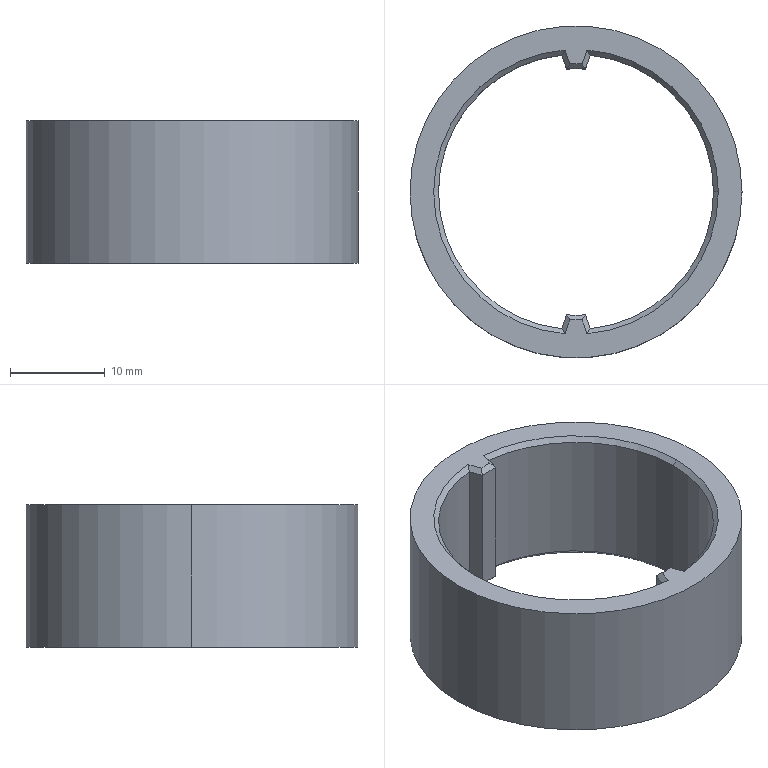Part | SolidWorks | features Chamfer 1, Extrusion 1, ICE 1 | 1 solid | 31 faces | box 35 x 35 x 15 mm | volume 4612 mm3 | plane 14 | cone 10 | cylinder 7 | commonest cylinder face diameters 29 x3 26 x2 35 x2
STEP:
#1=CARTESIAN_POINT('',(14.5,0.,14.5));
#2=VERTEX_POINT('',#1);
#3=CARTESIAN_POINT('',(1.5,14.422,14.5));
#4=VERTEX_POINT('',#3);
#5=CARTESIAN_POINT('',(0.,0.,14.5));
#6=DIRECTION('',(0.,0.,1.));
#7=DIRECTION('',(1.,0.,0.));
#8=AXIS2_PLACEMENT_3D('',#5,#6,#7);
#9=CIRCLE('',#8,14.5);
#10=EDGE_CURVE('',#2,#4,#9,.T.);
#11=ORIENTED_EDGE('',*,*,#10,.F.);
#12=CARTESIAN_POINT('',(15.,0.,15.));
#13=VERTEX_POINT('',#12);
#14=CARTESIAN_POINT('',(14.5,0.,14.5));
#15=DIRECTION('',(0.7071,0.,0.7071));
#16=VECTOR('',#15,1000.);
#17=LINE('',#14,#16);
#18=EDGE_CURVE('',#2,#13,#17,.T.);
#19=ORIENTED_EDGE('',*,*,#18,.T.);
#20=CARTESIAN_POINT('',(1.154,14.956,15.));
#21=VERTEX_POINT('',#20);
#22=CARTESIAN_POINT('',(0.,0.,15.));
#23=DIRECTION('',(0.,0.,-1.));
#24=DIRECTION('',(1.,0.,0.));
#25=AXIS2_PLACEMENT_3D('',#22,#23,#24);
#26=CIRCLE('',#25,15.);
#27=EDGE_CURVE('',#21,#13,#26,.T.);
#28=ORIENTED_EDGE('',*,*,#27,.F.);
#29=CARTESIAN_POINT('',(1.154,14.956,15.));
#30=CARTESIAN_POINT('',(1.27,14.779,14.833));
#31=CARTESIAN_POINT('',(1.386,14.601,14.666));
#32=CARTESIAN_POINT('',(1.5,14.422,14.5));
#33=B_SPLINE_CURVE_WITH_KNOTS('',3,(#29,#30,#31,#32),.UNSPECIFIED.,.F.,.F.,(4,4),(0.,0.0008088),.UNSPECIFIED.);
#34=EDGE_CURVE('',#21,#4,#33,.T.);
#35=ORIENTED_EDGE('',*,*,#34,.T.);
#36=EDGE_LOOP('',(#11,#19,#28,#35));
#37=FACE_OUTER_BOUND('',#36,.T.);
#38=CARTESIAN_POINT('',(0.,0.,14.5));
#39=DIRECTION('',(0.,0.,1.));
#40=DIRECTION('',(1.,0.,0.));
#41=AXIS2_PLACEMENT_3D('',#38,#39,#40);
#42=CONICAL_SURFACE('',#41,14.5,0.7854);
#43=ADVANCED_FACE('',(#37),#42,.F.);
#44=CARTESIAN_POINT('',(-14.5,0.,0.5));
#45=VERTEX_POINT('',#44);
#46=CARTESIAN_POINT('',(-1.5,14.422,0.5));
#47=VERTEX_POINT('',#46);
#48=CARTESIAN_POINT('',(0.,0.,0.5));
#49=DIRECTION('',(0.,0.,-1.));
#50=DIRECTION('',(1.,0.,0.));
#51=AXIS2_PLACEMENT_3D('',#48,#49,#50);
#52=CIRCLE('',#51,14.5);
#53=EDGE_CURVE('',#45,#47,#52,.T.);
#54=ORIENTED_EDGE('',*,*,#53,.F.);
#55=CARTESIAN_POINT('',(-15.,0.,0.));
#56=VERTEX_POINT('',#55);
#57=CARTESIAN_POINT('',(-15.,0.,0.));
#58=DIRECTION('',(-0.7071,0.,-0.7071));
#59=VECTOR('',#58,1000.);
#60=LINE('',#57,#59);
#61=EDGE_CURVE('',#45,#56,#60,.T.);
#62=ORIENTED_EDGE('',*,*,#61,.T.);
#63=CARTESIAN_POINT('',(-1.154,14.956,0.));
#64=VERTEX_POINT('',#63);
#65=CARTESIAN_POINT('',(0.,0.,0.));
#66=DIRECTION('',(0.,0.,1.));
#67=DIRECTION('',(1.,0.,0.));
#68=AXIS2_PLACEMENT_3D('',#65,#66,#67);
#69=CIRCLE('',#68,15.);
#70=EDGE_CURVE('',#64,#56,#69,.T.);
#71=ORIENTED_EDGE('',*,*,#70,.F.);
#72=CARTESIAN_POINT('',(-1.154,14.956,0.));
#73=CARTESIAN_POINT('',(-1.27,14.779,0.1672));
#74=CARTESIAN_POINT('',(-1.386,14.601,0.3339));
#75=CARTESIAN_POINT('',(-1.5,14.422,0.5));
#76=B_SPLINE_CURVE_WITH_KNOTS('',3,(#72,#73,#74,#75),.UNSPECIFIED.,.F.,.F.,(4,4),(0.,0.0008088),.UNSPECIFIED.);
#77=EDGE_CURVE('',#64,#47,#76,.T.);
#78=ORIENTED_EDGE('',*,*,#77,.T.);
#79=EDGE_LOOP('',(#54,#62,#71,#78));
#80=FACE_OUTER_BOUND('',#79,.T.);
#81=CARTESIAN_POINT('',(0.,0.,0.));
#82=DIRECTION('',(0.,0.,-1.));
#83=DIRECTION('',(-1.,0.,0.));
#84=AXIS2_PLACEMENT_3D('',#81,#82,#83);
#85=CONICAL_SURFACE('',#84,15.,0.7854);
#86=ADVANCED_FACE('',(#80),#85,.F.);
#87=CARTESIAN_POINT('',(17.5,0.,15.));
#88=VERTEX_POINT('',#87);
#89=CARTESIAN_POINT('',(-17.5,0.,15.));
#90=VERTEX_POINT('',#89);
#91=CARTESIAN_POINT('',(0.,0.,15.));
#92=DIRECTION('',(0.,0.,1.));
#93=DIRECTION('',(1.,0.,0.));
#94=AXIS2_PLACEMENT_3D('',#91,#92,#93);
#95=CIRCLE('',#94,17.5);
#96=EDGE_CURVE('',#88,#90,#95,.T.);
#97=ORIENTED_EDGE('',*,*,#96,.F.);
#98=CARTESIAN_POINT('',(17.5,0.,0.));
#99=VERTEX_POINT('',#98);
#100=CARTESIAN_POINT('',(17.5,0.,15.));
#101=DIRECTION('',(0.,0.,-1.));
#102=VECTOR('',#101,1000.);
#103=LINE('',#100,#102);
#104=EDGE_CURVE('',#88,#99,#103,.T.);
#105=ORIENTED_EDGE('',*,*,#104,.T.);
#106=CARTESIAN_POINT('',(-17.5,0.,0.));
#107=VERTEX_POINT('',#106);
#108=CARTESIAN_POINT('',(0.,0.,0.));
#109=DIRECTION('',(0.,0.,1.));
#110=DIRECTION('',(1.,0.,0.));
#111=AXIS2_PLACEMENT_3D('',#108,#109,#110);
#112=CIRCLE('',#111,17.5);
#113=EDGE_CURVE('',#99,#107,#112,.T.);
#114=ORIENTED_EDGE('',*,*,#113,.T.);
#115=CARTESIAN_POINT('',(-17.5,0.,15.));
#116=DIRECTION('',(0.,0.,-1.));
#117=VECTOR('',#116,1000.);
#118=LINE('',#115,#117);
#119=EDGE_CURVE('',#90,#107,#118,.T.);
#120=ORIENTED_EDGE('',*,*,#119,.F.);
#121=EDGE_LOOP('',(#97,#105,#114,#120));
#122=FACE_OUTER_BOUND('',#121,.T.);
#123=CARTESIAN_POINT('',(0.,0.,15.));
#124=DIRECTION('',(0.,0.,-1.));
#125=DIRECTION('',(-1.,0.,0.));
#126=AXIS2_PLACEMENT_3D('',#123,#124,#125);
#127=CYLINDRICAL_SURFACE('',#126,17.5);
#128=ADVANCED_FACE('',(#122),#127,.T.);
#129=CARTESIAN_POINT('',(-1.5,14.422,14.5));
#130=VERTEX_POINT('',#129);
#131=CARTESIAN_POINT('',(-14.5,0.,14.5));
#132=VERTEX_POINT('',#131);
#133=CARTESIAN_POINT('',(0.,0.,14.5));
#134=DIRECTION('',(0.,0.,1.));
#135=DIRECTION('',(1.,0.,0.));
#136=AXIS2_PLACEMENT_3D('',#133,#134,#135);
#137=CIRCLE('',#136,14.5);
#138=EDGE_CURVE('',#130,#132,#137,.T.);
#139=ORIENTED_EDGE('',*,*,#138,.T.);
#140=CARTESIAN_POINT('',(-14.5,0.,15.));
#141=DIRECTION('',(0.,0.,-1.));
#142=VECTOR('',#141,1000.);
#143=LINE('',#140,#142);
#144=EDGE_CURVE('',#132,#45,#143,.T.);
#145=ORIENTED_EDGE('',*,*,#144,.T.);
#146=ORIENTED_EDGE('',*,*,#53,.T.);
#147=CARTESIAN_POINT('',(-1.5,14.422,18.372));
#148=DIRECTION('',(0.,0.,-1.));
#149=VECTOR('',#148,1000.);
#150=LINE('',#147,#149);
#151=EDGE_CURVE('',#130,#47,#150,.T.);
#152=ORIENTED_EDGE('',*,*,#151,.F.);
#153=EDGE_LOOP('',(#139,#145,#146,#152));
#154=FACE_OUTER_BOUND('',#153,.T.);
#155=CARTESIAN_POINT('',(0.,0.,15.));
#156=DIRECTION('',(0.,0.,-1.));
#157=DIRECTION('',(-1.,0.,0.));
#158=AXIS2_PLACEMENT_3D('',#155,#156,#157);
#159=CYLINDRICAL_SURFACE('',#158,14.5);
#160=ADVANCED_FACE('',(#154),#159,.F.);
#161=CARTESIAN_POINT('',(1.5,14.422,0.5));
#162=VERTEX_POINT('',#161);
#163=CARTESIAN_POINT('',(1.5,14.422,18.372));
#164=DIRECTION('',(0.,0.,-1.));
#165=VECTOR('',#164,1000.);
#166=LINE('',#163,#165);
#167=EDGE_CURVE('',#4,#162,#166,.T.);
#168=ORIENTED_EDGE('',*,*,#167,.T.);
#169=CARTESIAN_POINT('',(1.5,-14.422,0.5));
#170=VERTEX_POINT('',#169);
#171=CARTESIAN_POINT('',(0.,0.,0.5));
#172=DIRECTION('',(0.,0.,-1.));
#173=DIRECTION('',(1.,0.,0.));
#174=AXIS2_PLACEMENT_3D('',#171,#172,#173);
#175=CIRCLE('',#174,14.5);
#176=EDGE_CURVE('',#162,#170,#175,.T.);
#177=ORIENTED_EDGE('',*,*,#176,.T.);
#178=CARTESIAN_POINT('',(1.5,-14.422,14.5));
#179=VERTEX_POINT('',#178);
#180=CARTESIAN_POINT('',(1.5,-14.422,18.372));
#181=DIRECTION('',(0.,0.,-1.));
#182=VECTOR('',#181,1000.);
#183=LINE('',#180,#182);
#184=EDGE_CURVE('',#179,#170,#183,.T.);
#185=ORIENTED_EDGE('',*,*,#184,.F.);
#186=CARTESIAN_POINT('',(0.,0.,14.5));
#187=DIRECTION('',(0.,0.,1.));
#188=DIRECTION('',(1.,0.,0.));
#189=AXIS2_PLACEMENT_3D('',#186,#187,#188);
#190=CIRCLE('',#189,14.5);
#191=EDGE_CURVE('',#179,#2,#190,.T.);
#192=ORIENTED_EDGE('',*,*,#191,.T.);
#193=ORIENTED_EDGE('',*,*,#10,.T.);
#194=EDGE_LOOP('',(#168,#177,#185,#192,#193));
#195=FACE_OUTER_BOUND('',#194,.T.);
#196=CARTESIAN_POINT('',(0.,0.,15.));
#197=DIRECTION('',(0.,0.,-1.));
#198=DIRECTION('',(-1.,0.,0.));
#199=AXIS2_PLACEMENT_3D('',#196,#197,#198);
#200=CYLINDRICAL_SURFACE('',#199,14.5);
#201=ADVANCED_FACE('',(#195),#200,.F.);
#202=ORIENTED_EDGE('',*,*,#144,.F.);
#203=CARTESIAN_POINT('',(-1.5,-14.422,14.5));
#204=VERTEX_POINT('',#203);
#205=CARTESIAN_POINT('',(0.,0.,14.5));
#206=DIRECTION('',(0.,0.,1.));
#207=DIRECTION('',(1.,0.,0.));
#208=AXIS2_PLACEMENT_3D('',#205,#206,#207);
#209=CIRCLE('',#208,14.5);
#210=EDGE_CURVE('',#132,#204,#209,.T.);
#211=ORIENTED_EDGE('',*,*,#210,.T.);
#212=CARTESIAN_POINT('',(-1.5,-14.422,0.5));
#213=VERTEX_POINT('',#212);
#214=CARTESIAN_POINT('',(-1.5,-14.422,18.372));
#215=DIRECTION('',(0.,0.,-1.));
#216=VECTOR('',#215,1000.);
#217=LINE('',#214,#216);
#218=EDGE_CURVE('',#204,#213,#217,.T.);
#219=ORIENTED_EDGE('',*,*,#218,.T.);
#220=CARTESIAN_POINT('',(0.,0.,0.5));
#221=DIRECTION('',(0.,0.,-1.));
#222=DIRECTION('',(1.,0.,0.));
#223=AXIS2_PLACEMENT_3D('',#220,#221,#222);
#224=CIRCLE('',#223,14.5);
#225=EDGE_CURVE('',#213,#45,#224,.T.);
#226=ORIENTED_EDGE('',*,*,#225,.T.);
#227=EDGE_LOOP('',(#202,#211,#219,#226));
#228=FACE_OUTER_BOUND('',#227,.T.);
#229=CARTESIAN_POINT('',(0.,0.,15.));
#230=DIRECTION('',(0.,0.,-1.));
#231=DIRECTION('',(-1.,0.,0.));
#232=AXIS2_PLACEMENT_3D('',#229,#230,#231);
#233=CYLINDRICAL_SURFACE('',#232,14.5);
#234=ADVANCED_FACE('',(#228),#233,.F.);
#235=CARTESIAN_POINT('',(1.154,-14.956,15.));
#236=VERTEX_POINT('',#235);
#237=CARTESIAN_POINT('',(0.6505,-13.484,15.));
#238=VERTEX_POINT('',#237);
#239=CARTESIAN_POINT('',(0.5269,-13.123,15.));
#240=DIRECTION('',(-0.3238,0.9461,0.));
#241=VECTOR('',#240,1000.);
#242=LINE('',#239,#241);
#243=EDGE_CURVE('',#236,#238,#242,.T.);
#244=ORIENTED_EDGE('',*,*,#243,.T.);
#245=CARTESIAN_POINT('',(-0.6505,-13.484,15.));
#246=VERTEX_POINT('',#245);
#247=CARTESIAN_POINT('',(0.,0.,15.));
#248=DIRECTION('',(0.,0.,-1.));
#249=DIRECTION('',(1.,0.,0.));
#250=AXIS2_PLACEMENT_3D('',#247,#248,#249);
#251=CIRCLE('',#250,13.5);
#252=EDGE_CURVE('',#238,#246,#251,.T.);
#253=ORIENTED_EDGE('',*,*,#252,.T.);
#254=CARTESIAN_POINT('',(-1.154,-14.956,15.));
#255=VERTEX_POINT('',#254);
#256=CARTESIAN_POINT('',(-1.027,-14.584,15.));
#257=DIRECTION('',(-0.3238,-0.9461,0.));
#258=VECTOR('',#257,1000.);
#259=LINE('',#256,#258);
#260=EDGE_CURVE('',#246,#255,#259,.T.);
#261=ORIENTED_EDGE('',*,*,#260,.T.);
#262=CARTESIAN_POINT('',(-1.154,14.956,15.));
#263=VERTEX_POINT('',#262);
#264=CARTESIAN_POINT('',(0.,0.,15.));
#265=DIRECTION('',(0.,0.,-1.));
#266=DIRECTION('',(1.,0.,0.));
#267=AXIS2_PLACEMENT_3D('',#264,#265,#266);
#268=CIRCLE('',#267,15.);
#269=EDGE_CURVE('',#255,#263,#268,.T.);
#270=ORIENTED_EDGE('',*,*,#269,.T.);
#271=CARTESIAN_POINT('',(-0.6505,13.484,15.));
#272=VERTEX_POINT('',#271);
#273=CARTESIAN_POINT('',(-0.5269,13.123,15.));
#274=DIRECTION('',(0.3238,-0.9461,0.));
#275=VECTOR('',#274,1000.);
#276=LINE('',#273,#275);
#277=EDGE_CURVE('',#263,#272,#276,.T.);
#278=ORIENTED_EDGE('',*,*,#277,.T.);
#279=CARTESIAN_POINT('',(0.6505,13.484,15.));
#280=VERTEX_POINT('',#279);
#281=CARTESIAN_POINT('',(0.,0.,15.));
#282=DIRECTION('',(0.,0.,-1.));
#283=DIRECTION('',(1.,0.,0.));
#284=AXIS2_PLACEMENT_3D('',#281,#282,#283);
#285=CIRCLE('',#284,13.5);
#286=EDGE_CURVE('',#272,#280,#285,.T.);
#287=ORIENTED_EDGE('',*,*,#286,.T.);
#288=CARTESIAN_POINT('',(1.027,14.584,15.));
#289=DIRECTION('',(0.3238,0.9461,0.));
#290=VECTOR('',#289,1000.);
#291=LINE('',#288,#290);
#292=EDGE_CURVE('',#280,#21,#291,.T.);
#293=ORIENTED_EDGE('',*,*,#292,.T.);
#294=ORIENTED_EDGE('',*,*,#27,.T.);
#295=CARTESIAN_POINT('',(0.,0.,15.));
#296=DIRECTION('',(0.,0.,-1.));
#297=DIRECTION('',(1.,0.,0.));
#298=AXIS2_PLACEMENT_3D('',#295,#296,#297);
#299=CIRCLE('',#298,15.);
#300=EDGE_CURVE('',#13,#236,#299,.T.);
#301=ORIENTED_EDGE('',*,*,#300,.T.);
#302=EDGE_LOOP('',(#244,#253,#261,#270,#278,#287,#293,#294,#301));
#303=FACE_BOUND('',#302,.T.);
#304=CARTESIAN_POINT('',(0.,0.,15.));
#305=DIRECTION('',(0.,0.,1.));
#306=DIRECTION('',(1.,0.,0.));
#307=AXIS2_PLACEMENT_3D('',#304,#305,#306);
#308=CIRCLE('',#307,17.5);
#309=EDGE_CURVE('',#90,#88,#308,.T.);
#310=ORIENTED_EDGE('',*,*,#309,.T.);
#311=ORIENTED_EDGE('',*,*,#96,.T.);
#312=EDGE_LOOP('',(#310,#311));
#313=FACE_OUTER_BOUND('',#312,.T.);
#314=CARTESIAN_POINT('',(0.,0.,15.));
#315=DIRECTION('',(0.,0.,1.));
#316=DIRECTION('',(1.,0.,0.));
#317=AXIS2_PLACEMENT_3D('',#314,#315,#316);
#318=PLANE('',#317);
#319=ADVANCED_FACE('',(#303,#313),#318,.T.);
#320=CARTESIAN_POINT('',(-1.154,-14.956,0.));
#321=VERTEX_POINT('',#320);
#322=CARTESIAN_POINT('',(-0.6505,-13.484,0.));
#323=VERTEX_POINT('',#322);
#324=CARTESIAN_POINT('',(3.549,-1.215,0.));
#325=DIRECTION('',(0.3238,0.9461,0.));
#326=VECTOR('',#325,1000.);
#327=LINE('',#324,#326);
#328=EDGE_CURVE('',#321,#323,#327,.T.);
#329=ORIENTED_EDGE('',*,*,#328,.T.);
#330=CARTESIAN_POINT('',(0.6505,-13.484,0.));
#331=VERTEX_POINT('',#330);
#332=CARTESIAN_POINT('',(0.,0.,0.));
#333=DIRECTION('',(0.,0.,1.));
#334=DIRECTION('',(1.,0.,0.));
#335=AXIS2_PLACEMENT_3D('',#332,#333,#334);
#336=CIRCLE('',#335,13.5);
#337=EDGE_CURVE('',#323,#331,#336,.T.);
#338=ORIENTED_EDGE('',*,*,#337,.T.);
#339=CARTESIAN_POINT('',(1.154,-14.956,0.));
#340=VERTEX_POINT('',#339);
#341=CARTESIAN_POINT('',(-3.549,-1.215,0.));
#342=DIRECTION('',(0.3238,-0.9461,0.));
#343=VECTOR('',#342,1000.);
#344=LINE('',#341,#343);
#345=EDGE_CURVE('',#331,#340,#344,.T.);
#346=ORIENTED_EDGE('',*,*,#345,.T.);
#347=CARTESIAN_POINT('',(1.154,14.956,0.));
#348=VERTEX_POINT('',#347);
#349=CARTESIAN_POINT('',(0.,0.,0.));
#350=DIRECTION('',(0.,0.,1.));
#351=DIRECTION('',(1.,0.,0.));
#352=AXIS2_PLACEMENT_3D('',#349,#350,#351);
#353=CIRCLE('',#352,15.);
#354=EDGE_CURVE('',#340,#348,#353,.T.);
#355=ORIENTED_EDGE('',*,*,#354,.T.);
#356=CARTESIAN_POINT('',(0.6505,13.484,0.));
#357=VERTEX_POINT('',#356);
#358=CARTESIAN_POINT('',(-3.549,1.215,0.));
#359=DIRECTION('',(-0.3238,-0.9461,0.));
#360=VECTOR('',#359,1000.);
#361=LINE('',#358,#360);
#362=EDGE_CURVE('',#348,#357,#361,.T.);
#363=ORIENTED_EDGE('',*,*,#362,.T.);
#364=CARTESIAN_POINT('',(-0.6505,13.484,0.));
#365=VERTEX_POINT('',#364);
#366=CARTESIAN_POINT('',(0.,0.,0.));
#367=DIRECTION('',(0.,0.,1.));
#368=DIRECTION('',(1.,0.,0.));
#369=AXIS2_PLACEMENT_3D('',#366,#367,#368);
#370=CIRCLE('',#369,13.5);
#371=EDGE_CURVE('',#357,#365,#370,.T.);
#372=ORIENTED_EDGE('',*,*,#371,.T.);
#373=CARTESIAN_POINT('',(3.549,1.215,0.));
#374=DIRECTION('',(-0.3238,0.9461,0.));
#375=VECTOR('',#374,1000.);
#376=LINE('',#373,#375);
#377=EDGE_CURVE('',#365,#64,#376,.T.);
#378=ORIENTED_EDGE('',*,*,#377,.T.);
#379=ORIENTED_EDGE('',*,*,#70,.T.);
#380=CARTESIAN_POINT('',(0.,0.,0.));
#381=DIRECTION('',(0.,0.,1.));
#382=DIRECTION('',(1.,0.,0.));
#383=AXIS2_PLACEMENT_3D('',#380,#381,#382);
#384=CIRCLE('',#383,15.);
#385=EDGE_CURVE('',#56,#321,#384,.T.);
#386=ORIENTED_EDGE('',*,*,#385,.T.);
#387=EDGE_LOOP('',(#329,#338,#346,#355,#363,#372,#378,#379,#386));
#388=FACE_BOUND('',#387,.T.);
#389=CARTESIAN_POINT('',(0.,0.,0.));
#390=DIRECTION('',(0.,0.,1.));
#391=DIRECTION('',(1.,0.,0.));
#392=AXIS2_PLACEMENT_3D('',#389,#390,#391);
#393=CIRCLE('',#392,17.5);
#394=EDGE_CURVE('',#107,#99,#393,.T.);
#395=ORIENTED_EDGE('',*,*,#394,.F.);
#396=ORIENTED_EDGE('',*,*,#113,.F.);
#397=EDGE_LOOP('',(#395,#396));
#398=FACE_OUTER_BOUND('',#397,.T.);
#399=CARTESIAN_POINT('',(0.,0.,0.));
#400=DIRECTION('',(0.,0.,1.));
#401=DIRECTION('',(1.,0.,0.));
#402=AXIS2_PLACEMENT_3D('',#399,#400,#401);
#403=PLANE('',#402);
#404=ADVANCED_FACE('',(#388,#398),#403,.F.);
#405=ORIENTED_EDGE('',*,*,#104,.F.);
#406=ORIENTED_EDGE('',*,*,#309,.F.);
#407=ORIENTED_EDGE('',*,*,#119,.T.);
#408=ORIENTED_EDGE('',*,*,#394,.T.);
#409=EDGE_LOOP('',(#405,#406,#407,#408));
#410=FACE_OUTER_BOUND('',#409,.T.);
#411=CARTESIAN_POINT('',(0.,0.,15.));
#412=DIRECTION('',(0.,0.,-1.));
#413=DIRECTION('',(-1.,0.,0.));
#414=AXIS2_PLACEMENT_3D('',#411,#412,#413);
#415=CYLINDRICAL_SURFACE('',#414,17.5);
#416=ADVANCED_FACE('',(#410),#415,.T.);
#417=ORIENTED_EDGE('',*,*,#151,.T.);
#418=CARTESIAN_POINT('',(-1.,12.961,0.5));
#419=VERTEX_POINT('',#418);
#420=CARTESIAN_POINT('',(-1.5,14.422,0.5));
#421=DIRECTION('',(0.3238,-0.9461,0.));
#422=VECTOR('',#421,1000.);
#423=LINE('',#420,#422);
#424=EDGE_CURVE('',#47,#419,#423,.T.);
#425=ORIENTED_EDGE('',*,*,#424,.T.);
#426=CARTESIAN_POINT('',(-1.,12.961,14.5));
#427=VERTEX_POINT('',#426);
#428=CARTESIAN_POINT('',(-1.,12.961,18.372));
#429=DIRECTION('',(0.,0.,-1.));
#430=VECTOR('',#429,1000.);
#431=LINE('',#428,#430);
#432=EDGE_CURVE('',#427,#419,#431,.T.);
#433=ORIENTED_EDGE('',*,*,#432,.F.);
#434=CARTESIAN_POINT('',(-1.5,14.422,14.5));
#435=DIRECTION('',(-0.3238,0.9461,0.));
#436=VECTOR('',#435,1000.);
#437=LINE('',#434,#436);
#438=EDGE_CURVE('',#427,#130,#437,.T.);
#439=ORIENTED_EDGE('',*,*,#438,.T.);
#440=EDGE_LOOP('',(#417,#425,#433,#439));
#441=FACE_OUTER_BOUND('',#440,.T.);
#442=CARTESIAN_POINT('',(-1.5,14.422,18.372));
#443=DIRECTION('',(0.9461,0.3238,0.));
#444=DIRECTION('',(-0.3238,0.9461,0.));
#445=AXIS2_PLACEMENT_3D('',#442,#443,#444);
#446=PLANE('',#445);
#447=ADVANCED_FACE('',(#441),#446,.F.);
#448=ORIENTED_EDGE('',*,*,#432,.T.);
#449=CARTESIAN_POINT('',(1.,12.961,0.5));
#450=VERTEX_POINT('',#449);
#451=CARTESIAN_POINT('',(0.,0.,0.5));
#452=DIRECTION('',(0.,0.,-1.));
#453=DIRECTION('',(1.,0.,0.));
#454=AXIS2_PLACEMENT_3D('',#451,#452,#453);
#455=CIRCLE('',#454,13.);
#456=EDGE_CURVE('',#419,#450,#455,.T.);
#457=ORIENTED_EDGE('',*,*,#456,.T.);
#458=CARTESIAN_POINT('',(1.,12.961,14.5));
#459=VERTEX_POINT('',#458);
#460=CARTESIAN_POINT('',(1.,12.961,18.372));
#461=DIRECTION('',(0.,0.,-1.));
#462=VECTOR('',#461,1000.);
#463=LINE('',#460,#462);
#464=EDGE_CURVE('',#459,#450,#463,.T.);
#465=ORIENTED_EDGE('',*,*,#464,.F.);
#466=CARTESIAN_POINT('',(0.,0.,14.5));
#467=DIRECTION('',(0.,0.,1.));
#468=DIRECTION('',(1.,0.,0.));
#469=AXIS2_PLACEMENT_3D('',#466,#467,#468);
#470=CIRCLE('',#469,13.);
#471=EDGE_CURVE('',#459,#427,#470,.T.);
#472=ORIENTED_EDGE('',*,*,#471,.T.);
#473=EDGE_LOOP('',(#448,#457,#465,#472));
#474=FACE_OUTER_BOUND('',#473,.T.);
#475=CARTESIAN_POINT('',(0.,0.,18.372));
#476=DIRECTION('',(0.,0.,-1.));
#477=DIRECTION('',(-1.,0.,0.));
#478=AXIS2_PLACEMENT_3D('',#475,#476,#477);
#479=CYLINDRICAL_SURFACE('',#478,13.);
#480=ADVANCED_FACE('',(#474),#479,.F.);
#481=ORIENTED_EDGE('',*,*,#464,.T.);
#482=CARTESIAN_POINT('',(1.,12.961,0.5));
#483=DIRECTION('',(0.3238,0.9461,0.));
#484=VECTOR('',#483,1000.);
#485=LINE('',#482,#484);
#486=EDGE_CURVE('',#450,#162,#485,.T.);
#487=ORIENTED_EDGE('',*,*,#486,.T.);
#488=ORIENTED_EDGE('',*,*,#167,.F.);
#489=CARTESIAN_POINT('',(1.,12.961,14.5));
#490=DIRECTION('',(-0.3238,-0.9461,0.));
#491=VECTOR('',#490,1000.);
#492=LINE('',#489,#491);
#493=EDGE_CURVE('',#4,#459,#492,.T.);
#494=ORIENTED_EDGE('',*,*,#493,.T.);
#495=EDGE_LOOP('',(#481,#487,#488,#494));
#496=FACE_OUTER_BOUND('',#495,.T.);
#497=CARTESIAN_POINT('',(1.,12.961,18.372));
#498=DIRECTION('',(-0.9461,0.3238,0.));
#499=DIRECTION('',(-0.3238,-0.9461,0.));
#500=AXIS2_PLACEMENT_3D('',#497,#498,#499);
#501=PLANE('',#500);
#502=ADVANCED_FACE('',(#496),#501,.F.);
#503=ORIENTED_EDGE('',*,*,#184,.T.);
#504=CARTESIAN_POINT('',(1.,-12.961,0.5));
#505=VERTEX_POINT('',#504);
#506=CARTESIAN_POINT('',(1.,-12.961,0.5));
#507=DIRECTION('',(-0.3238,0.9461,0.));
#508=VECTOR('',#507,1000.);
#509=LINE('',#506,#508);
#510=EDGE_CURVE('',#170,#505,#509,.T.);
#511=ORIENTED_EDGE('',*,*,#510,.T.);
#512=CARTESIAN_POINT('',(1.,-12.961,14.5));
#513=VERTEX_POINT('',#512);
#514=CARTESIAN_POINT('',(1.,-12.961,18.372));
#515=DIRECTION('',(0.,0.,-1.));
#516=VECTOR('',#515,1000.);
#517=LINE('',#514,#516);
#518=EDGE_CURVE('',#513,#505,#517,.T.);
#519=ORIENTED_EDGE('',*,*,#518,.F.);
#520=CARTESIAN_POINT('',(1.5,-14.422,14.5));
#521=DIRECTION('',(0.3238,-0.9461,0.));
#522=VECTOR('',#521,1000.);
#523=LINE('',#520,#522);
#524=EDGE_CURVE('',#513,#179,#523,.T.);
#525=ORIENTED_EDGE('',*,*,#524,.T.);
#526=EDGE_LOOP('',(#503,#511,#519,#525));
#527=FACE_OUTER_BOUND('',#526,.T.);
#528=CARTESIAN_POINT('',(1.,-12.961,18.372));
#529=DIRECTION('',(-0.9461,-0.3238,0.));
#530=DIRECTION('',(0.3238,-0.9461,0.));
#531=AXIS2_PLACEMENT_3D('',#528,#529,#530);
#532=PLANE('',#531);
#533=ADVANCED_FACE('',(#527),#532,.F.);
#534=ORIENTED_EDGE('',*,*,#518,.T.);
#535=CARTESIAN_POINT('',(-1.,-12.961,0.5));
#536=VERTEX_POINT('',#535);
#537=CARTESIAN_POINT('',(0.,0.,0.5));
#538=DIRECTION('',(0.,0.,-1.));
#539=DIRECTION('',(1.,0.,0.));
#540=AXIS2_PLACEMENT_3D('',#537,#538,#539);
#541=CIRCLE('',#540,13.);
#542=EDGE_CURVE('',#505,#536,#541,.T.);
#543=ORIENTED_EDGE('',*,*,#542,.T.);
#544=CARTESIAN_POINT('',(-1.,-12.961,14.5));
#545=VERTEX_POINT('',#544);
#546=CARTESIAN_POINT('',(-1.,-12.961,18.372));
#547=DIRECTION('',(0.,0.,-1.));
#548=VECTOR('',#547,1000.);
#549=LINE('',#546,#548);
#550=EDGE_CURVE('',#545,#536,#549,.T.);
#551=ORIENTED_EDGE('',*,*,#550,.F.);
#552=CARTESIAN_POINT('',(0.,0.,14.5));
#553=DIRECTION('',(0.,0.,1.));
#554=DIRECTION('',(1.,0.,0.));
#555=AXIS2_PLACEMENT_3D('',#552,#553,#554);
#556=CIRCLE('',#555,13.);
#557=EDGE_CURVE('',#545,#513,#556,.T.);
#558=ORIENTED_EDGE('',*,*,#557,.T.);
#559=EDGE_LOOP('',(#534,#543,#551,#558));
#560=FACE_OUTER_BOUND('',#559,.T.);
#561=CARTESIAN_POINT('',(0.,0.,18.372));
#562=DIRECTION('',(0.,0.,-1.));
#563=DIRECTION('',(-1.,0.,0.));
#564=AXIS2_PLACEMENT_3D('',#561,#562,#563);
#565=CYLINDRICAL_SURFACE('',#564,13.);
#566=ADVANCED_FACE('',(#560),#565,.F.);
#567=ORIENTED_EDGE('',*,*,#550,.T.);
#568=CARTESIAN_POINT('',(-1.5,-14.422,0.5));
#569=DIRECTION('',(-0.3238,-0.9461,0.));
#570=VECTOR('',#569,1000.);
#571=LINE('',#568,#570);
#572=EDGE_CURVE('',#536,#213,#571,.T.);
#573=ORIENTED_EDGE('',*,*,#572,.T.);
#574=ORIENTED_EDGE('',*,*,#218,.F.);
#575=CARTESIAN_POINT('',(-1.,-12.961,14.5));
#576=DIRECTION('',(0.3238,0.9461,0.));
#577=VECTOR('',#576,1000.);
#578=LINE('',#575,#577);
#579=EDGE_CURVE('',#204,#545,#578,.T.);
#580=ORIENTED_EDGE('',*,*,#579,.T.);
#581=EDGE_LOOP('',(#567,#573,#574,#580));
#582=FACE_OUTER_BOUND('',#581,.T.);
#583=CARTESIAN_POINT('',(-1.5,-14.422,18.372));
#584=DIRECTION('',(0.9461,-0.3238,0.));
#585=DIRECTION('',(0.3238,0.9461,0.));
#586=AXIS2_PLACEMENT_3D('',#583,#584,#585);
#587=PLANE('',#586);
#588=ADVANCED_FACE('',(#582),#587,.F.);
#589=CARTESIAN_POINT('',(-0.6505,13.484,0.));
#590=CARTESIAN_POINT('',(-0.768,13.311,0.1672));
#591=CARTESIAN_POINT('',(-0.8845,13.137,0.3339));
#592=CARTESIAN_POINT('',(-1.,12.961,0.5));
#593=B_SPLINE_CURVE_WITH_KNOTS('',3,(#589,#590,#591,#592),.UNSPECIFIED.,.F.,.F.,(4,4),(0.,0.0008034),.UNSPECIFIED.);
#594=EDGE_CURVE('',#365,#419,#593,.T.);
#595=ORIENTED_EDGE('',*,*,#594,.F.);
#596=ORIENTED_EDGE('',*,*,#371,.F.);
#597=CARTESIAN_POINT('',(1.,12.961,0.5));
#598=CARTESIAN_POINT('',(0.8845,13.137,0.3339));
#599=CARTESIAN_POINT('',(0.768,13.311,0.1672));
#600=CARTESIAN_POINT('',(0.6505,13.484,0.));
#601=B_SPLINE_CURVE_WITH_KNOTS('',3,(#597,#598,#599,#600),.UNSPECIFIED.,.F.,.F.,(4,4),(0.,0.0008034),.UNSPECIFIED.);
#602=EDGE_CURVE('',#450,#357,#601,.T.);
#603=ORIENTED_EDGE('',*,*,#602,.F.);
#604=ORIENTED_EDGE('',*,*,#456,.F.);
#605=EDGE_LOOP('',(#595,#596,#603,#604));
#606=FACE_OUTER_BOUND('',#605,.T.);
#607=CARTESIAN_POINT('',(0.,0.,0.5));
#608=DIRECTION('',(0.,0.,-1.));
#609=DIRECTION('',(-1.,0.,0.));
#610=AXIS2_PLACEMENT_3D('',#607,#608,#609);
#611=CONICAL_SURFACE('',#610,13.,0.7854);
#612=ADVANCED_FACE('',(#606),#611,.F.);
#613=ORIENTED_EDGE('',*,*,#602,.T.);
#614=ORIENTED_EDGE('',*,*,#362,.F.);
#615=CARTESIAN_POINT('',(1.5,14.422,0.5));
#616=CARTESIAN_POINT('',(1.386,14.601,0.3339));
#617=CARTESIAN_POINT('',(1.27,14.779,0.1672));
#618=CARTESIAN_POINT('',(1.154,14.956,0.));
#619=B_SPLINE_CURVE_WITH_KNOTS('',3,(#615,#616,#617,#618),.UNSPECIFIED.,.F.,.F.,(4,4),(0.,0.0008088),.UNSPECIFIED.);
#620=EDGE_CURVE('',#162,#348,#619,.T.);
#621=ORIENTED_EDGE('',*,*,#620,.F.);
#622=ORIENTED_EDGE('',*,*,#486,.F.);
#623=EDGE_LOOP('',(#613,#614,#621,#622));
#624=FACE_OUTER_BOUND('',#623,.T.);
#625=CARTESIAN_POINT('',(1.,12.961,0.5));
#626=DIRECTION('',(-0.669,0.229,0.7071));
#627=DIRECTION('',(0.3238,0.9461,0.));
#628=AXIS2_PLACEMENT_3D('',#625,#626,#627);
#629=PLANE('',#628);
#630=ADVANCED_FACE('',(#624),#629,.F.);
#631=ORIENTED_EDGE('',*,*,#594,.T.);
#632=ORIENTED_EDGE('',*,*,#424,.F.);
#633=ORIENTED_EDGE('',*,*,#77,.F.);
#634=ORIENTED_EDGE('',*,*,#377,.F.);
#635=EDGE_LOOP('',(#631,#632,#633,#634));
#636=FACE_OUTER_BOUND('',#635,.T.);
#637=CARTESIAN_POINT('',(-1.5,14.422,0.5));
#638=DIRECTION('',(0.669,0.229,0.7071));
#639=DIRECTION('',(0.3238,-0.9461,0.));
#640=AXIS2_PLACEMENT_3D('',#637,#638,#639);
#641=PLANE('',#640);
#642=ADVANCED_FACE('',(#636),#641,.F.);
#643=ORIENTED_EDGE('',*,*,#620,.T.);
#644=ORIENTED_EDGE('',*,*,#354,.F.);
#645=CARTESIAN_POINT('',(1.5,-14.422,0.5));
#646=CARTESIAN_POINT('',(1.386,-14.601,0.3339));
#647=CARTESIAN_POINT('',(1.27,-14.779,0.1672));
#648=CARTESIAN_POINT('',(1.154,-14.956,0.));
#649=B_SPLINE_CURVE_WITH_KNOTS('',3,(#645,#646,#647,#648),.UNSPECIFIED.,.F.,.F.,(4,4),(0.,0.0008088),.UNSPECIFIED.);
#650=EDGE_CURVE('',#170,#340,#649,.T.);
#651=ORIENTED_EDGE('',*,*,#650,.F.);
#652=ORIENTED_EDGE('',*,*,#176,.F.);
#653=EDGE_LOOP('',(#643,#644,#651,#652));
#654=FACE_OUTER_BOUND('',#653,.T.);
#655=CARTESIAN_POINT('',(0.,0.,0.));
#656=DIRECTION('',(0.,0.,-1.));
#657=DIRECTION('',(-1.,0.,0.));
#658=AXIS2_PLACEMENT_3D('',#655,#656,#657);
#659=CONICAL_SURFACE('',#658,15.,0.7854);
#660=ADVANCED_FACE('',(#654),#659,.F.);
#661=ORIENTED_EDGE('',*,*,#61,.F.);
#662=ORIENTED_EDGE('',*,*,#225,.F.);
#663=CARTESIAN_POINT('',(-1.154,-14.956,0.));
#664=CARTESIAN_POINT('',(-1.27,-14.779,0.1672));
#665=CARTESIAN_POINT('',(-1.386,-14.601,0.3339));
#666=CARTESIAN_POINT('',(-1.5,-14.422,0.5));
#667=B_SPLINE_CURVE_WITH_KNOTS('',3,(#663,#664,#665,#666),.UNSPECIFIED.,.F.,.F.,(4,4),(0.,0.0008088),.UNSPECIFIED.);
#668=EDGE_CURVE('',#321,#213,#667,.T.);
#669=ORIENTED_EDGE('',*,*,#668,.F.);
#670=ORIENTED_EDGE('',*,*,#385,.F.);
#671=EDGE_LOOP('',(#661,#662,#669,#670));
#672=FACE_OUTER_BOUND('',#671,.T.);
#673=CARTESIAN_POINT('',(0.,0.,0.));
#674=DIRECTION('',(0.,0.,-1.));
#675=DIRECTION('',(-1.,0.,0.));
#676=AXIS2_PLACEMENT_3D('',#673,#674,#675);
#677=CONICAL_SURFACE('',#676,15.,0.7854);
#678=ADVANCED_FACE('',(#672),#677,.F.);
#679=ORIENTED_EDGE('',*,*,#650,.T.);
#680=ORIENTED_EDGE('',*,*,#345,.F.);
#681=CARTESIAN_POINT('',(1.,-12.961,0.5));
#682=CARTESIAN_POINT('',(0.8845,-13.137,0.3339));
#683=CARTESIAN_POINT('',(0.768,-13.311,0.1672));
#684=CARTESIAN_POINT('',(0.6505,-13.484,0.));
#685=B_SPLINE_CURVE_WITH_KNOTS('',3,(#681,#682,#683,#684),.UNSPECIFIED.,.F.,.F.,(4,4),(0.,0.0008034),.UNSPECIFIED.);
#686=EDGE_CURVE('',#505,#331,#685,.T.);
#687=ORIENTED_EDGE('',*,*,#686,.F.);
#688=ORIENTED_EDGE('',*,*,#510,.F.);
#689=EDGE_LOOP('',(#679,#680,#687,#688));
#690=FACE_OUTER_BOUND('',#689,.T.);
#691=CARTESIAN_POINT('',(1.,-12.961,0.5));
#692=DIRECTION('',(-0.669,-0.229,0.7071));
#693=DIRECTION('',(-0.3238,0.9461,0.));
#694=AXIS2_PLACEMENT_3D('',#691,#692,#693);
#695=PLANE('',#694);
#696=ADVANCED_FACE('',(#690),#695,.F.);
#697=ORIENTED_EDGE('',*,*,#668,.T.);
#698=ORIENTED_EDGE('',*,*,#572,.F.);
#699=CARTESIAN_POINT('',(-0.6505,-13.484,0.));
#700=CARTESIAN_POINT('',(-0.768,-13.311,0.1672));
#701=CARTESIAN_POINT('',(-0.8845,-13.137,0.3339));
#702=CARTESIAN_POINT('',(-1.,-12.961,0.5));
#703=B_SPLINE_CURVE_WITH_KNOTS('',3,(#699,#700,#701,#702),.UNSPECIFIED.,.F.,.F.,(4,4),(0.,0.0008034),.UNSPECIFIED.);
#704=EDGE_CURVE('',#323,#536,#703,.T.);
#705=ORIENTED_EDGE('',*,*,#704,.F.);
#706=ORIENTED_EDGE('',*,*,#328,.F.);
#707=EDGE_LOOP('',(#697,#698,#705,#706));
#708=FACE_OUTER_BOUND('',#707,.T.);
#709=CARTESIAN_POINT('',(-1.5,-14.422,0.5));
#710=DIRECTION('',(0.669,-0.229,0.7071));
#711=DIRECTION('',(-0.3238,-0.9461,0.));
#712=AXIS2_PLACEMENT_3D('',#709,#710,#711);
#713=PLANE('',#712);
#714=ADVANCED_FACE('',(#708),#713,.F.);
#715=ORIENTED_EDGE('',*,*,#686,.T.);
#716=ORIENTED_EDGE('',*,*,#337,.F.);
#717=ORIENTED_EDGE('',*,*,#704,.T.);
#718=ORIENTED_EDGE('',*,*,#542,.F.);
#719=EDGE_LOOP('',(#715,#716,#717,#718));
#720=FACE_OUTER_BOUND('',#719,.T.);
#721=CARTESIAN_POINT('',(0.,0.,0.5));
#722=DIRECTION('',(0.,0.,-1.));
#723=DIRECTION('',(-1.,0.,0.));
#724=AXIS2_PLACEMENT_3D('',#721,#722,#723);
#725=CONICAL_SURFACE('',#724,13.,0.7854);
#726=ADVANCED_FACE('',(#720),#725,.F.);
#727=CARTESIAN_POINT('',(-1.,12.961,14.5));
#728=CARTESIAN_POINT('',(-0.8845,13.137,14.666));
#729=CARTESIAN_POINT('',(-0.768,13.311,14.833));
#730=CARTESIAN_POINT('',(-0.6505,13.484,15.));
#731=B_SPLINE_CURVE_WITH_KNOTS('',3,(#727,#728,#729,#730),.UNSPECIFIED.,.F.,.F.,(4,4),(0.,0.0008034),.UNSPECIFIED.);
#732=EDGE_CURVE('',#427,#272,#731,.T.);
#733=ORIENTED_EDGE('',*,*,#732,.F.);
#734=ORIENTED_EDGE('',*,*,#471,.F.);
#735=CARTESIAN_POINT('',(0.6505,13.484,15.));
#736=CARTESIAN_POINT('',(0.768,13.311,14.833));
#737=CARTESIAN_POINT('',(0.8845,13.137,14.666));
#738=CARTESIAN_POINT('',(1.,12.961,14.5));
#739=B_SPLINE_CURVE_WITH_KNOTS('',3,(#735,#736,#737,#738),.UNSPECIFIED.,.F.,.F.,(4,4),(0.,0.0008034),.UNSPECIFIED.);
#740=EDGE_CURVE('',#280,#459,#739,.T.);
#741=ORIENTED_EDGE('',*,*,#740,.F.);
#742=ORIENTED_EDGE('',*,*,#286,.F.);
#743=EDGE_LOOP('',(#733,#734,#741,#742));
#744=FACE_OUTER_BOUND('',#743,.T.);
#745=CARTESIAN_POINT('',(0.,0.,15.));
#746=DIRECTION('',(0.,0.,1.));
#747=DIRECTION('',(1.,0.,0.));
#748=AXIS2_PLACEMENT_3D('',#745,#746,#747);
#749=CONICAL_SURFACE('',#748,13.5,0.7854);
#750=ADVANCED_FACE('',(#744),#749,.F.);
#751=ORIENTED_EDGE('',*,*,#740,.T.);
#752=ORIENTED_EDGE('',*,*,#493,.F.);
#753=ORIENTED_EDGE('',*,*,#34,.F.);
#754=ORIENTED_EDGE('',*,*,#292,.F.);
#755=EDGE_LOOP('',(#751,#752,#753,#754));
#756=FACE_OUTER_BOUND('',#755,.T.);
#757=CARTESIAN_POINT('',(-3.549,1.215,15.));
#758=DIRECTION('',(0.669,-0.229,0.7071));
#759=DIRECTION('',(-0.3238,-0.9461,0.));
#760=AXIS2_PLACEMENT_3D('',#757,#758,#759);
#761=PLANE('',#760);
#762=ADVANCED_FACE('',(#756),#761,.T.);
#763=ORIENTED_EDGE('',*,*,#732,.T.);
#764=ORIENTED_EDGE('',*,*,#277,.F.);
#765=CARTESIAN_POINT('',(-1.5,14.422,14.5));
#766=CARTESIAN_POINT('',(-1.386,14.601,14.666));
#767=CARTESIAN_POINT('',(-1.27,14.779,14.833));
#768=CARTESIAN_POINT('',(-1.154,14.956,15.));
#769=B_SPLINE_CURVE_WITH_KNOTS('',3,(#765,#766,#767,#768),.UNSPECIFIED.,.F.,.F.,(4,4),(0.,0.0008088),.UNSPECIFIED.);
#770=EDGE_CURVE('',#130,#263,#769,.T.);
#771=ORIENTED_EDGE('',*,*,#770,.F.);
#772=ORIENTED_EDGE('',*,*,#438,.F.);
#773=EDGE_LOOP('',(#763,#764,#771,#772));
#774=FACE_OUTER_BOUND('',#773,.T.);
#775=CARTESIAN_POINT('',(3.549,1.215,15.));
#776=DIRECTION('',(-0.669,-0.229,0.7071));
#777=DIRECTION('',(-0.3238,0.9461,0.));
#778=AXIS2_PLACEMENT_3D('',#775,#776,#777);
#779=PLANE('',#778);
#780=ADVANCED_FACE('',(#774),#779,.T.);
#781=ORIENTED_EDGE('',*,*,#18,.F.);
#782=ORIENTED_EDGE('',*,*,#191,.F.);
#783=CARTESIAN_POINT('',(1.154,-14.956,15.));
#784=CARTESIAN_POINT('',(1.27,-14.779,14.833));
#785=CARTESIAN_POINT('',(1.386,-14.601,14.666));
#786=CARTESIAN_POINT('',(1.5,-14.422,14.5));
#787=B_SPLINE_CURVE_WITH_KNOTS('',3,(#783,#784,#785,#786),.UNSPECIFIED.,.F.,.F.,(4,4),(0.,0.0008088),.UNSPECIFIED.);
#788=EDGE_CURVE('',#236,#179,#787,.T.);
#789=ORIENTED_EDGE('',*,*,#788,.F.);
#790=ORIENTED_EDGE('',*,*,#300,.F.);
#791=EDGE_LOOP('',(#781,#782,#789,#790));
#792=FACE_OUTER_BOUND('',#791,.T.);
#793=CARTESIAN_POINT('',(0.,0.,14.5));
#794=DIRECTION('',(0.,0.,1.));
#795=DIRECTION('',(1.,0.,0.));
#796=AXIS2_PLACEMENT_3D('',#793,#794,#795);
#797=CONICAL_SURFACE('',#796,14.5,0.7854);
#798=ADVANCED_FACE('',(#792),#797,.F.);
#799=ORIENTED_EDGE('',*,*,#770,.T.);
#800=ORIENTED_EDGE('',*,*,#269,.F.);
#801=CARTESIAN_POINT('',(-1.5,-14.422,14.5));
#802=CARTESIAN_POINT('',(-1.386,-14.601,14.666));
#803=CARTESIAN_POINT('',(-1.27,-14.779,14.833));
#804=CARTESIAN_POINT('',(-1.154,-14.956,15.));
#805=B_SPLINE_CURVE_WITH_KNOTS('',3,(#801,#802,#803,#804),.UNSPECIFIED.,.F.,.F.,(4,4),(0.,0.0008088),.UNSPECIFIED.);
#806=EDGE_CURVE('',#204,#255,#805,.T.);
#807=ORIENTED_EDGE('',*,*,#806,.F.);
#808=ORIENTED_EDGE('',*,*,#210,.F.);
#809=ORIENTED_EDGE('',*,*,#138,.F.);
#810=EDGE_LOOP('',(#799,#800,#807,#808,#809));
#811=FACE_OUTER_BOUND('',#810,.T.);
#812=CARTESIAN_POINT('',(0.,0.,14.5));
#813=DIRECTION('',(0.,0.,1.));
#814=DIRECTION('',(1.,0.,0.));
#815=AXIS2_PLACEMENT_3D('',#812,#813,#814);
#816=CONICAL_SURFACE('',#815,14.5,0.7854);
#817=ADVANCED_FACE('',(#811),#816,.F.);
#818=ORIENTED_EDGE('',*,*,#788,.T.);
#819=ORIENTED_EDGE('',*,*,#524,.F.);
#820=CARTESIAN_POINT('',(0.6505,-13.484,15.));
#821=CARTESIAN_POINT('',(0.768,-13.311,14.833));
#822=CARTESIAN_POINT('',(0.8845,-13.137,14.666));
#823=CARTESIAN_POINT('',(1.,-12.961,14.5));
#824=B_SPLINE_CURVE_WITH_KNOTS('',3,(#820,#821,#822,#823),.UNSPECIFIED.,.F.,.F.,(4,4),(0.,0.0008034),.UNSPECIFIED.);
#825=EDGE_CURVE('',#238,#513,#824,.T.);
#826=ORIENTED_EDGE('',*,*,#825,.F.);
#827=ORIENTED_EDGE('',*,*,#243,.F.);
#828=EDGE_LOOP('',(#818,#819,#826,#827));
#829=FACE_OUTER_BOUND('',#828,.T.);
#830=CARTESIAN_POINT('',(-3.549,-1.215,15.));
#831=DIRECTION('',(0.669,0.229,0.7071));
#832=DIRECTION('',(0.3238,-0.9461,0.));
#833=AXIS2_PLACEMENT_3D('',#830,#831,#832);
#834=PLANE('',#833);
#835=ADVANCED_FACE('',(#829),#834,.T.);
#836=ORIENTED_EDGE('',*,*,#806,.T.);
#837=ORIENTED_EDGE('',*,*,#260,.F.);
#838=CARTESIAN_POINT('',(-1.,-12.961,14.5));
#839=CARTESIAN_POINT('',(-0.8845,-13.137,14.666));
#840=CARTESIAN_POINT('',(-0.768,-13.311,14.833));
#841=CARTESIAN_POINT('',(-0.6505,-13.484,15.));
#842=B_SPLINE_CURVE_WITH_KNOTS('',3,(#838,#839,#840,#841),.UNSPECIFIED.,.F.,.F.,(4,4),(0.,0.0008034),.UNSPECIFIED.);
#843=EDGE_CURVE('',#545,#246,#842,.T.);
#844=ORIENTED_EDGE('',*,*,#843,.F.);
#845=ORIENTED_EDGE('',*,*,#579,.F.);
#846=EDGE_LOOP('',(#836,#837,#844,#845));
#847=FACE_OUTER_BOUND('',#846,.T.);
#848=CARTESIAN_POINT('',(3.549,-1.215,15.));
#849=DIRECTION('',(-0.669,0.229,0.7071));
#850=DIRECTION('',(0.3238,0.9461,0.));
#851=AXIS2_PLACEMENT_3D('',#848,#849,#850);
#852=PLANE('',#851);
#853=ADVANCED_FACE('',(#847),#852,.T.);
#854=ORIENTED_EDGE('',*,*,#825,.T.);
#855=ORIENTED_EDGE('',*,*,#557,.F.);
#856=ORIENTED_EDGE('',*,*,#843,.T.);
#857=ORIENTED_EDGE('',*,*,#252,.F.);
#858=EDGE_LOOP('',(#854,#855,#856,#857));
#859=FACE_OUTER_BOUND('',#858,.T.);
#860=CARTESIAN_POINT('',(0.,0.,15.));
#861=DIRECTION('',(0.,0.,1.));
#862=DIRECTION('',(1.,0.,0.));
#863=AXIS2_PLACEMENT_3D('',#860,#861,#862);
#864=CONICAL_SURFACE('',#863,13.5,0.7854);
#865=ADVANCED_FACE('',(#859),#864,.F.);
#866=CLOSED_SHELL('',(#43,#86,#128,#160,#201,#234,#319,#404,#416,#447,#480,#502,#533,#566,#588,#612,#630,#642,#660,#678,#696,#714,#726,#750,#762,#780,#798,#817,#835,#853,#865));
#867=MANIFOLD_SOLID_BREP('',#866);
#868=CARTESIAN_POINT('',(0.,0.,0.));
#869=DIRECTION('',(0.,0.,1.));
#870=DIRECTION('',(1.,0.,0.));
#871=AXIS2_PLACEMENT_3D('',#868,#869,#870);
#872=(LENGTH_UNIT()NAMED_UNIT(*)SI_UNIT(.MILLI.,.METRE.));
#873=UNCERTAINTY_MEASURE_WITH_UNIT(LENGTH_MEASURE(0.00001),#872,'','');
#874=(NAMED_UNIT(*)PLANE_ANGLE_UNIT()SI_UNIT($,.RADIAN.));
#875=(NAMED_UNIT(*)SI_UNIT($,.STERADIAN.)SOLID_ANGLE_UNIT());
#876=(GEOMETRIC_REPRESENTATION_CONTEXT(3)GLOBAL_UNCERTAINTY_ASSIGNED_CONTEXT((#873))GLOBAL_UNIT_ASSIGNED_CONTEXT((#872,#874,#875))REPRESENTATION_CONTEXT('',''));
#877=ADVANCED_BREP_SHAPE_REPRESENTATION('',(#867,#871),#876);